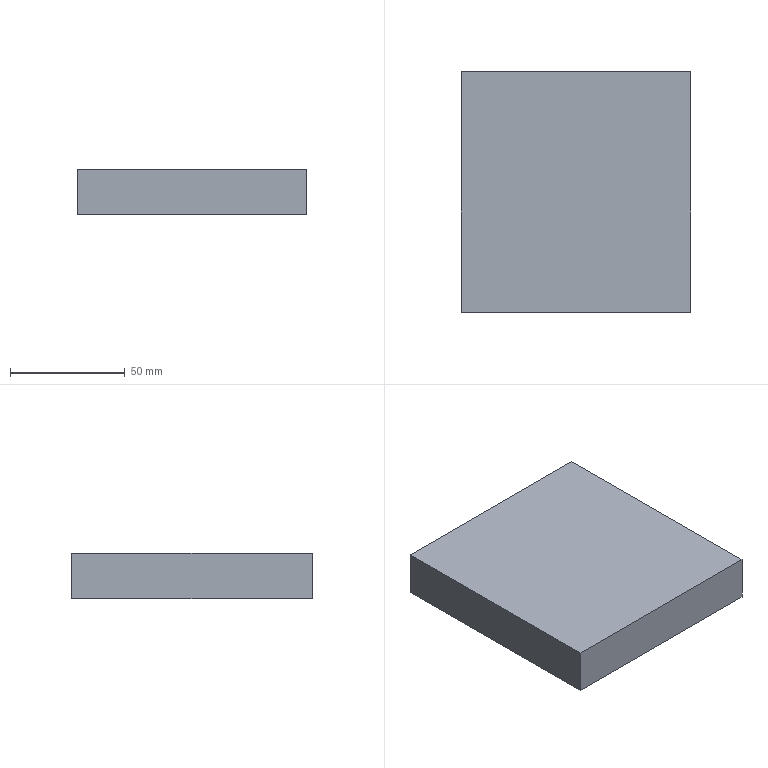Part | SolidWorks | features BaseBody 1 | 1 solid | 6 faces | box 100 x 105 x 20 mm | volume 210000 mm3 | plane 6
STEP:
#1=CARTESIAN_POINT('',(50.,-52.5,0.));
#2=VERTEX_POINT('',#1);
#3=CARTESIAN_POINT('',(50.,52.5,0.));
#4=VERTEX_POINT('',#3);
#5=CARTESIAN_POINT('',(50.,-52.5,0.));
#6=DIRECTION('',(0.,1.,0.));
#7=VECTOR('',#6,1000.);
#8=LINE('',#5,#7);
#9=EDGE_CURVE('',#2,#4,#8,.T.);
#10=ORIENTED_EDGE('',*,*,#9,.T.);
#11=CARTESIAN_POINT('',(50.,52.5,20.));
#12=VERTEX_POINT('',#11);
#13=CARTESIAN_POINT('',(50.,52.5,20.));
#14=DIRECTION('',(0.,0.,-1.));
#15=VECTOR('',#14,1000.);
#16=LINE('',#13,#15);
#17=EDGE_CURVE('',#12,#4,#16,.T.);
#18=ORIENTED_EDGE('',*,*,#17,.F.);
#19=CARTESIAN_POINT('',(50.,-52.5,20.));
#20=VERTEX_POINT('',#19);
#21=CARTESIAN_POINT('',(50.,-52.5,20.));
#22=DIRECTION('',(0.,1.,0.));
#23=VECTOR('',#22,1000.);
#24=LINE('',#21,#23);
#25=EDGE_CURVE('',#20,#12,#24,.T.);
#26=ORIENTED_EDGE('',*,*,#25,.F.);
#27=CARTESIAN_POINT('',(50.,-52.5,20.));
#28=DIRECTION('',(0.,0.,-1.));
#29=VECTOR('',#28,1000.);
#30=LINE('',#27,#29);
#31=EDGE_CURVE('',#20,#2,#30,.T.);
#32=ORIENTED_EDGE('',*,*,#31,.T.);
#33=EDGE_LOOP('',(#10,#18,#26,#32));
#34=FACE_OUTER_BOUND('',#33,.T.);
#35=CARTESIAN_POINT('',(50.,-52.5,20.));
#36=DIRECTION('',(-1.,0.,0.));
#37=DIRECTION('',(0.,0.,1.));
#38=AXIS2_PLACEMENT_3D('',#35,#36,#37);
#39=PLANE('',#38);
#40=ADVANCED_FACE('',(#34),#39,.F.);
#41=CARTESIAN_POINT('',(-50.,52.5,0.));
#42=VERTEX_POINT('',#41);
#43=CARTESIAN_POINT('',(-50.,52.5,0.));
#44=DIRECTION('',(-1.,0.,0.));
#45=VECTOR('',#44,1000.);
#46=LINE('',#43,#45);
#47=EDGE_CURVE('',#4,#42,#46,.T.);
#48=ORIENTED_EDGE('',*,*,#47,.T.);
#49=CARTESIAN_POINT('',(-50.,52.5,20.));
#50=VERTEX_POINT('',#49);
#51=CARTESIAN_POINT('',(-50.,52.5,20.));
#52=DIRECTION('',(0.,0.,-1.));
#53=VECTOR('',#52,1000.);
#54=LINE('',#51,#53);
#55=EDGE_CURVE('',#50,#42,#54,.T.);
#56=ORIENTED_EDGE('',*,*,#55,.F.);
#57=CARTESIAN_POINT('',(-50.,52.5,20.));
#58=DIRECTION('',(-1.,0.,0.));
#59=VECTOR('',#58,1000.);
#60=LINE('',#57,#59);
#61=EDGE_CURVE('',#12,#50,#60,.T.);
#62=ORIENTED_EDGE('',*,*,#61,.F.);
#63=ORIENTED_EDGE('',*,*,#17,.T.);
#64=EDGE_LOOP('',(#48,#56,#62,#63));
#65=FACE_OUTER_BOUND('',#64,.T.);
#66=CARTESIAN_POINT('',(-50.,52.5,20.));
#67=DIRECTION('',(0.,-1.,0.));
#68=DIRECTION('',(0.,0.,-1.));
#69=AXIS2_PLACEMENT_3D('',#66,#67,#68);
#70=PLANE('',#69);
#71=ADVANCED_FACE('',(#65),#70,.F.);
#72=CARTESIAN_POINT('',(-50.,-52.5,0.));
#73=VERTEX_POINT('',#72);
#74=CARTESIAN_POINT('',(-50.,-52.5,0.));
#75=DIRECTION('',(0.,-1.,0.));
#76=VECTOR('',#75,1000.);
#77=LINE('',#74,#76);
#78=EDGE_CURVE('',#42,#73,#77,.T.);
#79=ORIENTED_EDGE('',*,*,#78,.T.);
#80=CARTESIAN_POINT('',(-50.,-52.5,20.));
#81=VERTEX_POINT('',#80);
#82=CARTESIAN_POINT('',(-50.,-52.5,20.));
#83=DIRECTION('',(0.,0.,-1.));
#84=VECTOR('',#83,1000.);
#85=LINE('',#82,#84);
#86=EDGE_CURVE('',#81,#73,#85,.T.);
#87=ORIENTED_EDGE('',*,*,#86,.F.);
#88=CARTESIAN_POINT('',(-50.,-52.5,20.));
#89=DIRECTION('',(0.,-1.,0.));
#90=VECTOR('',#89,1000.);
#91=LINE('',#88,#90);
#92=EDGE_CURVE('',#50,#81,#91,.T.);
#93=ORIENTED_EDGE('',*,*,#92,.F.);
#94=ORIENTED_EDGE('',*,*,#55,.T.);
#95=EDGE_LOOP('',(#79,#87,#93,#94));
#96=FACE_OUTER_BOUND('',#95,.T.);
#97=CARTESIAN_POINT('',(-50.,-52.5,20.));
#98=DIRECTION('',(1.,0.,0.));
#99=DIRECTION('',(0.,0.,-1.));
#100=AXIS2_PLACEMENT_3D('',#97,#98,#99);
#101=PLANE('',#100);
#102=ADVANCED_FACE('',(#96),#101,.F.);
#103=CARTESIAN_POINT('',(-50.,-52.5,0.));
#104=DIRECTION('',(1.,0.,0.));
#105=VECTOR('',#104,1000.);
#106=LINE('',#103,#105);
#107=EDGE_CURVE('',#73,#2,#106,.T.);
#108=ORIENTED_EDGE('',*,*,#107,.T.);
#109=ORIENTED_EDGE('',*,*,#31,.F.);
#110=CARTESIAN_POINT('',(-50.,-52.5,20.));
#111=DIRECTION('',(1.,0.,0.));
#112=VECTOR('',#111,1000.);
#113=LINE('',#110,#112);
#114=EDGE_CURVE('',#81,#20,#113,.T.);
#115=ORIENTED_EDGE('',*,*,#114,.F.);
#116=ORIENTED_EDGE('',*,*,#86,.T.);
#117=EDGE_LOOP('',(#108,#109,#115,#116));
#118=FACE_OUTER_BOUND('',#117,.T.);
#119=CARTESIAN_POINT('',(-50.,-52.5,20.));
#120=DIRECTION('',(0.,1.,0.));
#121=DIRECTION('',(0.,0.,1.));
#122=AXIS2_PLACEMENT_3D('',#119,#120,#121);
#123=PLANE('',#122);
#124=ADVANCED_FACE('',(#118),#123,.F.);
#125=ORIENTED_EDGE('',*,*,#25,.T.);
#126=ORIENTED_EDGE('',*,*,#61,.T.);
#127=ORIENTED_EDGE('',*,*,#92,.T.);
#128=ORIENTED_EDGE('',*,*,#114,.T.);
#129=EDGE_LOOP('',(#125,#126,#127,#128));
#130=FACE_OUTER_BOUND('',#129,.T.);
#131=CARTESIAN_POINT('',(0.,0.,20.));
#132=DIRECTION('',(0.,0.,-1.));
#133=DIRECTION('',(-1.,0.,0.));
#134=AXIS2_PLACEMENT_3D('',#131,#132,#133);
#135=PLANE('',#134);
#136=ADVANCED_FACE('',(#130),#135,.F.);
#137=ORIENTED_EDGE('',*,*,#9,.F.);
#138=ORIENTED_EDGE('',*,*,#107,.F.);
#139=ORIENTED_EDGE('',*,*,#78,.F.);
#140=ORIENTED_EDGE('',*,*,#47,.F.);
#141=EDGE_LOOP('',(#137,#138,#139,#140));
#142=FACE_OUTER_BOUND('',#141,.T.);
#143=CARTESIAN_POINT('',(0.,0.,0.));
#144=DIRECTION('',(0.,0.,-1.));
#145=DIRECTION('',(-1.,0.,0.));
#146=AXIS2_PLACEMENT_3D('',#143,#144,#145);
#147=PLANE('',#146);
#148=ADVANCED_FACE('',(#142),#147,.T.);
#149=CLOSED_SHELL('',(#40,#71,#102,#124,#136,#148));
#150=MANIFOLD_SOLID_BREP('',#149);
#151=CARTESIAN_POINT('',(0.,0.,0.));
#152=DIRECTION('',(0.,0.,1.));
#153=DIRECTION('',(1.,0.,0.));
#154=AXIS2_PLACEMENT_3D('',#151,#152,#153);
#155=(LENGTH_UNIT()NAMED_UNIT(*)SI_UNIT(.MILLI.,.METRE.));
#156=UNCERTAINTY_MEASURE_WITH_UNIT(LENGTH_MEASURE(0.00001),#155,'','');
#157=(NAMED_UNIT(*)PLANE_ANGLE_UNIT()SI_UNIT($,.RADIAN.));
#158=(NAMED_UNIT(*)SI_UNIT($,.STERADIAN.)SOLID_ANGLE_UNIT());
#159=(GEOMETRIC_REPRESENTATION_CONTEXT(3)GLOBAL_UNCERTAINTY_ASSIGNED_CONTEXT((#156))GLOBAL_UNIT_ASSIGNED_CONTEXT((#155,#157,#158))REPRESENTATION_CONTEXT('',''));
#160=ADVANCED_BREP_SHAPE_REPRESENTATION('',(#150,#154),#159);